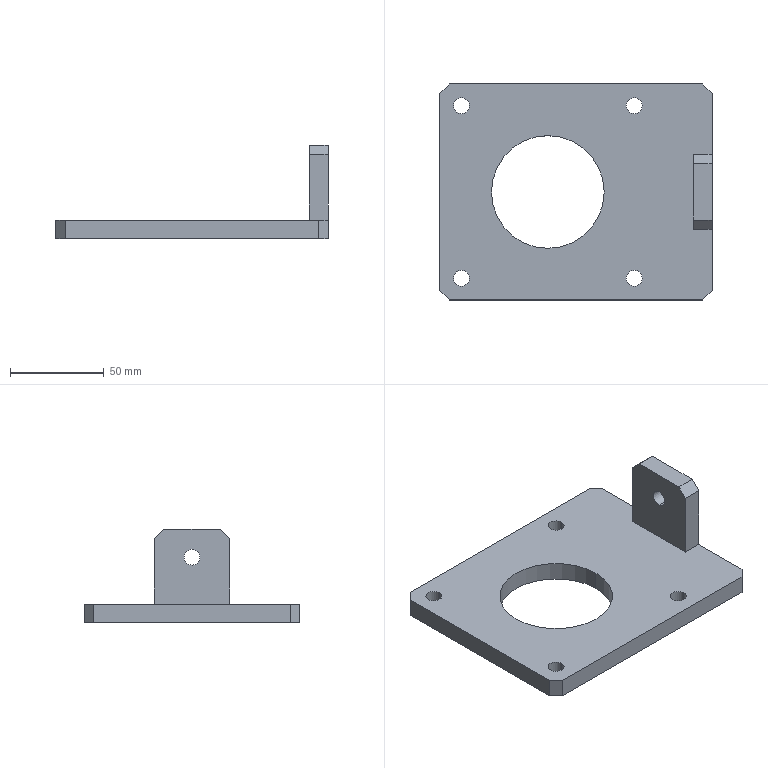Part | STEP file | PN_0056_adjusting plate_default_machined_ | 2 solids | 30 faces | box 145 x 115 x 50 mm | volume 150888 mm3 | plane 18 | cylinder 12 | commonest cylinder face diameters 8.5 x10 60 x2